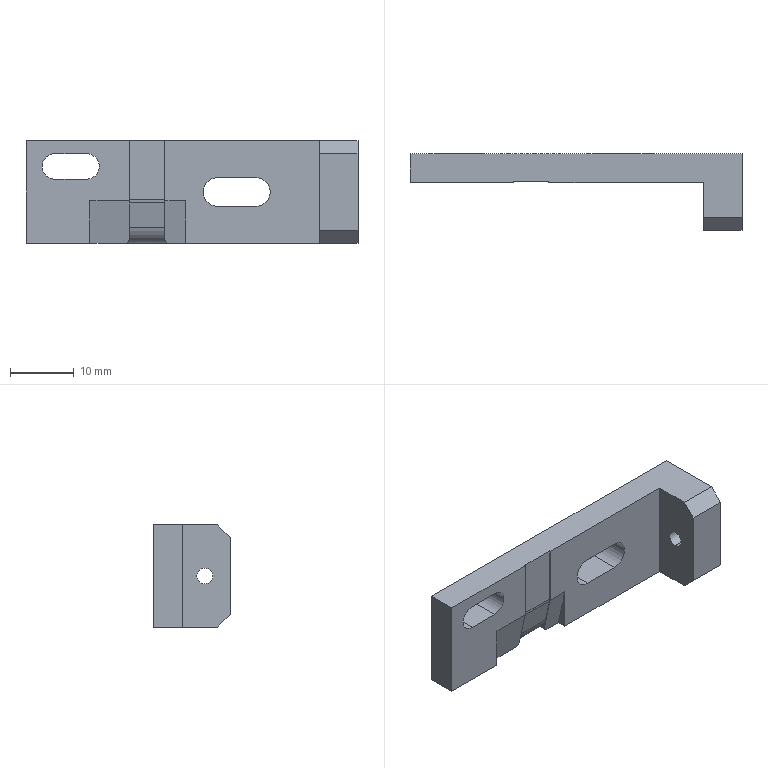Part | SolidWorks | features ICE 6, Chamfer 2, Fillet 2, 3DProfileFeature 1, Extrusion 1, HoleWzd 1 | 1 solid | 33 faces | box 52 x 12 x 16 mm | volume 3986 mm3 | plane 25 | cylinder 8 | commonest cylinder face diameters 4 x3 2.5 x2 4.5 x2 6 x1
STEP:
#1=CARTESIAN_POINT('',(23.,-3.5,1.25));
#2=VERTEX_POINT('',#1);
#3=CARTESIAN_POINT('',(23.,-3.5,-1.25));
#4=VERTEX_POINT('',#3);
#5=CARTESIAN_POINT('',(23.,-3.5,0.));
#6=DIRECTION('',(1.,0.,0.));
#7=DIRECTION('',(0.,0.,-1.));
#8=AXIS2_PLACEMENT_3D('',#5,#6,#7);
#9=CIRCLE('',#8,1.25);
#10=EDGE_CURVE('',#2,#4,#9,.T.);
#11=ORIENTED_EDGE('',*,*,#10,.F.);
#12=CARTESIAN_POINT('',(29.,-3.5,1.25));
#13=VERTEX_POINT('',#12);
#14=CARTESIAN_POINT('',(29.,-3.5,1.25));
#15=DIRECTION('',(1.,0.,0.));
#16=VECTOR('',#15,1000.);
#17=LINE('',#14,#16);
#18=EDGE_CURVE('',#2,#13,#17,.T.);
#19=ORIENTED_EDGE('',*,*,#18,.T.);
#20=CARTESIAN_POINT('',(29.,-3.5,-1.25));
#21=VERTEX_POINT('',#20);
#22=CARTESIAN_POINT('',(29.,-3.5,0.));
#23=DIRECTION('',(1.,0.,0.));
#24=DIRECTION('',(0.,0.,-1.));
#25=AXIS2_PLACEMENT_3D('',#22,#23,#24);
#26=CIRCLE('',#25,1.25);
#27=EDGE_CURVE('',#13,#21,#26,.T.);
#28=ORIENTED_EDGE('',*,*,#27,.T.);
#29=CARTESIAN_POINT('',(29.,-3.5,-1.25));
#30=DIRECTION('',(1.,0.,0.));
#31=VECTOR('',#30,1000.);
#32=LINE('',#29,#31);
#33=EDGE_CURVE('',#4,#21,#32,.T.);
#34=ORIENTED_EDGE('',*,*,#33,.F.);
#35=EDGE_LOOP('',(#11,#19,#28,#34));
#36=FACE_OUTER_BOUND('',#35,.T.);
#37=CARTESIAN_POINT('',(29.,-3.5,0.));
#38=DIRECTION('',(1.,0.,0.));
#39=DIRECTION('',(0.,0.,-1.));
#40=AXIS2_PLACEMENT_3D('',#37,#38,#39);
#41=CYLINDRICAL_SURFACE('',#40,1.25);
#42=ADVANCED_FACE('',(#36),#41,.F.);
#43=CARTESIAN_POINT('',(-13.5,0.,2.));
#44=VERTEX_POINT('',#43);
#45=CARTESIAN_POINT('',(-18.5,0.,2.));
#46=VERTEX_POINT('',#45);
#47=CARTESIAN_POINT('',(0.,0.,2.));
#48=DIRECTION('',(-1.,0.,0.));
#49=VECTOR('',#48,1000.);
#50=LINE('',#47,#49);
#51=EDGE_CURVE('',#44,#46,#50,.T.);
#52=ORIENTED_EDGE('',*,*,#51,.T.);
#53=CARTESIAN_POINT('',(-18.5,0.,6.));
#54=VERTEX_POINT('',#53);
#55=CARTESIAN_POINT('',(-18.5,0.,4.));
#56=DIRECTION('',(0.,1.,0.));
#57=DIRECTION('',(0.,0.,1.));
#58=AXIS2_PLACEMENT_3D('',#55,#56,#57);
#59=CIRCLE('',#58,2.);
#60=EDGE_CURVE('',#46,#54,#59,.T.);
#61=ORIENTED_EDGE('',*,*,#60,.T.);
#62=CARTESIAN_POINT('',(-13.5,0.,6.));
#63=VERTEX_POINT('',#62);
#64=CARTESIAN_POINT('',(0.,0.,6.));
#65=DIRECTION('',(1.,0.,0.));
#66=VECTOR('',#65,1000.);
#67=LINE('',#64,#66);
#68=EDGE_CURVE('',#54,#63,#67,.T.);
#69=ORIENTED_EDGE('',*,*,#68,.T.);
#70=CARTESIAN_POINT('',(-13.5,0.,4.));
#71=DIRECTION('',(0.,1.,0.));
#72=DIRECTION('',(0.,0.,1.));
#73=AXIS2_PLACEMENT_3D('',#70,#71,#72);
#74=CIRCLE('',#73,2.);
#75=EDGE_CURVE('',#63,#44,#74,.T.);
#76=ORIENTED_EDGE('',*,*,#75,.T.);
#77=EDGE_LOOP('',(#52,#61,#69,#76));
#78=FACE_BOUND('',#77,.T.);
#79=CARTESIAN_POINT('',(-6.75,0.,8.));
#80=VERTEX_POINT('',#79);
#81=CARTESIAN_POINT('',(-6.75,0.,-1.4));
#82=VERTEX_POINT('',#81);
#83=CARTESIAN_POINT('',(-6.75,0.,0.));
#84=DIRECTION('',(0.,0.,-1.));
#85=VECTOR('',#84,1000.);
#86=LINE('',#83,#85);
#87=EDGE_CURVE('',#80,#82,#86,.T.);
#88=ORIENTED_EDGE('',*,*,#87,.F.);
#89=CARTESIAN_POINT('',(-23.,0.,8.));
#90=VERTEX_POINT('',#89);
#91=CARTESIAN_POINT('',(-23.,0.,8.));
#92=DIRECTION('',(1.,0.,0.));
#93=VECTOR('',#92,1000.);
#94=LINE('',#91,#93);
#95=EDGE_CURVE('',#90,#80,#94,.T.);
#96=ORIENTED_EDGE('',*,*,#95,.F.);
#97=CARTESIAN_POINT('',(-23.,0.,-8.));
#98=VERTEX_POINT('',#97);
#99=CARTESIAN_POINT('',(-23.,0.,-8.));
#100=DIRECTION('',(0.,0.,1.));
#101=VECTOR('',#100,1000.);
#102=LINE('',#99,#101);
#103=EDGE_CURVE('',#98,#90,#102,.T.);
#104=ORIENTED_EDGE('',*,*,#103,.F.);
#105=CARTESIAN_POINT('',(-13.,0.,-8.));
#106=VERTEX_POINT('',#105);
#107=CARTESIAN_POINT('',(-23.,0.,-8.));
#108=DIRECTION('',(-1.,0.,0.));
#109=VECTOR('',#108,1000.);
#110=LINE('',#107,#109);
#111=EDGE_CURVE('',#106,#98,#110,.T.);
#112=ORIENTED_EDGE('',*,*,#111,.F.);
#113=CARTESIAN_POINT('',(-13.,0.,-1.4));
#114=VERTEX_POINT('',#113);
#115=CARTESIAN_POINT('',(-13.,0.,0.));
#116=DIRECTION('',(0.,0.,1.));
#117=VECTOR('',#116,1000.);
#118=LINE('',#115,#117);
#119=EDGE_CURVE('',#106,#114,#118,.T.);
#120=ORIENTED_EDGE('',*,*,#119,.T.);
#121=CARTESIAN_POINT('',(2.,0.,-1.4));
#122=DIRECTION('',(-1.,0.,0.));
#123=VECTOR('',#122,1000.);
#124=LINE('',#121,#123);
#125=EDGE_CURVE('',#82,#114,#124,.T.);
#126=ORIENTED_EDGE('',*,*,#125,.F.);
#127=EDGE_LOOP('',(#88,#96,#104,#112,#120,#126));
#128=FACE_OUTER_BOUND('',#127,.T.);
#129=CARTESIAN_POINT('',(0.,0.,0.));
#130=DIRECTION('',(0.,1.,0.));
#131=DIRECTION('',(0.,0.,1.));
#132=AXIS2_PLACEMENT_3D('',#129,#130,#131);
#133=PLANE('',#132);
#134=ADVANCED_FACE('',(#78,#128),#133,.F.);
#135=CARTESIAN_POINT('',(-7.25,1.403,-8.));
#136=VERTEX_POINT('',#135);
#137=CARTESIAN_POINT('',(-13.,1.403,-8.));
#138=VERTEX_POINT('',#137);
#139=CARTESIAN_POINT('',(-23.,1.403,-8.));
#140=DIRECTION('',(-1.,0.,0.));
#141=VECTOR('',#140,1000.);
#142=LINE('',#139,#141);
#143=EDGE_CURVE('',#136,#138,#142,.T.);
#144=ORIENTED_EDGE('',*,*,#143,.F.);
#145=CARTESIAN_POINT('',(-6.75,1.297,-7.5));
#146=VERTEX_POINT('',#145);
#147=CARTESIAN_POINT('',(-7.572,1.471,-8.322));
#148=DIRECTION('',(0.6993,-0.1486,0.6993));
#149=VECTOR('',#148,1000.);
#150=LINE('',#147,#149);
#151=EDGE_CURVE('',#136,#146,#150,.T.);
#152=ORIENTED_EDGE('',*,*,#151,.T.);
#153=CARTESIAN_POINT('',(-6.75,0.,-1.4));
#154=DIRECTION('',(0.,0.2079,-0.9781));
#155=VECTOR('',#154,1000.);
#156=LINE('',#153,#155);
#157=EDGE_CURVE('',#82,#146,#156,.T.);
#158=ORIENTED_EDGE('',*,*,#157,.F.);
#159=ORIENTED_EDGE('',*,*,#125,.T.);
#160=CARTESIAN_POINT('',(-13.,0.,-1.4));
#161=DIRECTION('',(0.,0.2079,-0.9781));
#162=VECTOR('',#161,1000.);
#163=LINE('',#160,#162);
#164=EDGE_CURVE('',#114,#138,#163,.T.);
#165=ORIENTED_EDGE('',*,*,#164,.T.);
#166=EDGE_LOOP('',(#144,#152,#158,#159,#165));
#167=FACE_OUTER_BOUND('',#166,.T.);
#168=CARTESIAN_POINT('',(2.,0.,-1.4));
#169=DIRECTION('',(0.,0.9781,0.2079));
#170=DIRECTION('',(0.,-0.2079,0.9781));
#171=AXIS2_PLACEMENT_3D('',#168,#169,#170);
#172=PLANE('',#171);
#173=ADVANCED_FACE('',(#167),#172,.F.);
#174=CARTESIAN_POINT('',(-0.75,3.934,-8.));
#175=VERTEX_POINT('',#174);
#176=CARTESIAN_POINT('',(-7.25,3.934,-8.));
#177=VERTEX_POINT('',#176);
#178=CARTESIAN_POINT('',(-23.,3.934,-8.));
#179=DIRECTION('',(-1.,0.,0.));
#180=VECTOR('',#179,1000.);
#181=LINE('',#178,#180);
#182=EDGE_CURVE('',#175,#177,#181,.T.);
#183=ORIENTED_EDGE('',*,*,#182,.T.);
#184=CARTESIAN_POINT('',(-7.25,1.403,-8.));
#185=DIRECTION('',(0.,-1.,0.));
#186=VECTOR('',#185,1000.);
#187=LINE('',#184,#186);
#188=EDGE_CURVE('',#177,#136,#187,.T.);
#189=ORIENTED_EDGE('',*,*,#188,.T.);
#190=ORIENTED_EDGE('',*,*,#143,.T.);
#191=CARTESIAN_POINT('',(-13.,4.5,-8.));
#192=DIRECTION('',(0.,-1.,0.));
#193=VECTOR('',#192,1000.);
#194=LINE('',#191,#193);
#195=EDGE_CURVE('',#138,#106,#194,.T.);
#196=ORIENTED_EDGE('',*,*,#195,.T.);
#197=ORIENTED_EDGE('',*,*,#111,.T.);
#198=CARTESIAN_POINT('',(-23.,4.5,-8.));
#199=VERTEX_POINT('',#198);
#200=CARTESIAN_POINT('',(-23.,4.5,-8.));
#201=DIRECTION('',(0.,-1.,0.));
#202=VECTOR('',#201,1000.);
#203=LINE('',#200,#202);
#204=EDGE_CURVE('',#199,#98,#203,.T.);
#205=ORIENTED_EDGE('',*,*,#204,.F.);
#206=CARTESIAN_POINT('',(29.,4.5,-8.));
#207=VERTEX_POINT('',#206);
#208=CARTESIAN_POINT('',(-23.,4.5,-8.));
#209=DIRECTION('',(-1.,0.,0.));
#210=VECTOR('',#209,1000.);
#211=LINE('',#208,#210);
#212=EDGE_CURVE('',#207,#199,#211,.T.);
#213=ORIENTED_EDGE('',*,*,#212,.F.);
#214=CARTESIAN_POINT('',(29.,-5.5,-8.));
#215=VERTEX_POINT('',#214);
#216=CARTESIAN_POINT('',(29.,4.5,-8.));
#217=DIRECTION('',(0.,1.,0.));
#218=VECTOR('',#217,1000.);
#219=LINE('',#216,#218);
#220=EDGE_CURVE('',#215,#207,#219,.T.);
#221=ORIENTED_EDGE('',*,*,#220,.F.);
#222=CARTESIAN_POINT('',(23.,-5.5,-8.));
#223=VERTEX_POINT('',#222);
#224=CARTESIAN_POINT('',(-23.,-5.5,-8.));
#225=DIRECTION('',(-1.,0.,0.));
#226=VECTOR('',#225,1000.);
#227=LINE('',#224,#226);
#228=EDGE_CURVE('',#215,#223,#227,.T.);
#229=ORIENTED_EDGE('',*,*,#228,.T.);
#230=CARTESIAN_POINT('',(23.,0.,-8.));
#231=VERTEX_POINT('',#230);
#232=CARTESIAN_POINT('',(23.,4.5,-8.));
#233=DIRECTION('',(0.,1.,0.));
#234=VECTOR('',#233,1000.);
#235=LINE('',#232,#234);
#236=EDGE_CURVE('',#223,#231,#235,.T.);
#237=ORIENTED_EDGE('',*,*,#236,.T.);
#238=CARTESIAN_POINT('',(2.,0.,-8.));
#239=VERTEX_POINT('',#238);
#240=CARTESIAN_POINT('',(-23.,0.,-8.));
#241=DIRECTION('',(-1.,0.,0.));
#242=VECTOR('',#241,1000.);
#243=LINE('',#240,#242);
#244=EDGE_CURVE('',#231,#239,#243,.T.);
#245=ORIENTED_EDGE('',*,*,#244,.T.);
#246=CARTESIAN_POINT('',(2.,1.403,-8.));
#247=VERTEX_POINT('',#246);
#248=CARTESIAN_POINT('',(2.,4.5,-8.));
#249=DIRECTION('',(0.,-1.,0.));
#250=VECTOR('',#249,1000.);
#251=LINE('',#248,#250);
#252=EDGE_CURVE('',#247,#239,#251,.T.);
#253=ORIENTED_EDGE('',*,*,#252,.F.);
#254=CARTESIAN_POINT('',(-0.75,1.403,-8.));
#255=VERTEX_POINT('',#254);
#256=CARTESIAN_POINT('',(-23.,1.403,-8.));
#257=DIRECTION('',(-1.,0.,0.));
#258=VECTOR('',#257,1000.);
#259=LINE('',#256,#258);
#260=EDGE_CURVE('',#247,#255,#259,.T.);
#261=ORIENTED_EDGE('',*,*,#260,.T.);
#262=CARTESIAN_POINT('',(-0.75,4.5,-8.));
#263=DIRECTION('',(0.,1.,0.));
#264=VECTOR('',#263,1000.);
#265=LINE('',#262,#264);
#266=EDGE_CURVE('',#255,#175,#265,.T.);
#267=ORIENTED_EDGE('',*,*,#266,.T.);
#268=EDGE_LOOP('',(#183,#189,#190,#196,#197,#205,#213,#221,#229,#237,#245,#253,#261,#267));
#269=FACE_OUTER_BOUND('',#268,.T.);
#270=CARTESIAN_POINT('',(-23.,4.5,-8.));
#271=DIRECTION('',(0.,0.,1.));
#272=DIRECTION('',(1.,0.,0.));
#273=AXIS2_PLACEMENT_3D('',#270,#271,#272);
#274=PLANE('',#273);
#275=ADVANCED_FACE('',(#269),#274,.F.);
#276=CARTESIAN_POINT('',(13.,0.,-2.25));
#277=VERTEX_POINT('',#276);
#278=CARTESIAN_POINT('',(7.,0.,-2.25));
#279=VERTEX_POINT('',#278);
#280=CARTESIAN_POINT('',(0.,0.,-2.25));
#281=DIRECTION('',(-1.,0.,0.));
#282=VECTOR('',#281,1000.);
#283=LINE('',#280,#282);
#284=EDGE_CURVE('',#277,#279,#283,.T.);
#285=ORIENTED_EDGE('',*,*,#284,.T.);
#286=CARTESIAN_POINT('',(7.,0.,2.25));
#287=VERTEX_POINT('',#286);
#288=CARTESIAN_POINT('',(7.,0.,0.));
#289=DIRECTION('',(0.,1.,0.));
#290=DIRECTION('',(0.,0.,1.));
#291=AXIS2_PLACEMENT_3D('',#288,#289,#290);
#292=CIRCLE('',#291,2.25);
#293=EDGE_CURVE('',#279,#287,#292,.T.);
#294=ORIENTED_EDGE('',*,*,#293,.T.);
#295=CARTESIAN_POINT('',(13.,0.,2.25));
#296=VERTEX_POINT('',#295);
#297=CARTESIAN_POINT('',(0.,0.,2.25));
#298=DIRECTION('',(1.,0.,0.));
#299=VECTOR('',#298,1000.);
#300=LINE('',#297,#299);
#301=EDGE_CURVE('',#287,#296,#300,.T.);
#302=ORIENTED_EDGE('',*,*,#301,.T.);
#303=CARTESIAN_POINT('',(13.,0.,0.));
#304=DIRECTION('',(0.,1.,0.));
#305=DIRECTION('',(0.,0.,1.));
#306=AXIS2_PLACEMENT_3D('',#303,#304,#305);
#307=CIRCLE('',#306,2.25);
#308=EDGE_CURVE('',#296,#277,#307,.T.);
#309=ORIENTED_EDGE('',*,*,#308,.T.);
#310=EDGE_LOOP('',(#285,#294,#302,#309));
#311=FACE_BOUND('',#310,.T.);
#312=CARTESIAN_POINT('',(-1.25,0.,8.));
#313=VERTEX_POINT('',#312);
#314=CARTESIAN_POINT('',(23.,0.,8.));
#315=VERTEX_POINT('',#314);
#316=CARTESIAN_POINT('',(-23.,0.,8.));
#317=DIRECTION('',(1.,0.,0.));
#318=VECTOR('',#317,1000.);
#319=LINE('',#316,#318);
#320=EDGE_CURVE('',#313,#315,#319,.T.);
#321=ORIENTED_EDGE('',*,*,#320,.F.);
#322=CARTESIAN_POINT('',(-1.25,0.,-1.4));
#323=VERTEX_POINT('',#322);
#324=CARTESIAN_POINT('',(-1.25,0.,0.));
#325=DIRECTION('',(0.,0.,-1.));
#326=VECTOR('',#325,1000.);
#327=LINE('',#324,#326);
#328=EDGE_CURVE('',#313,#323,#327,.T.);
#329=ORIENTED_EDGE('',*,*,#328,.T.);
#330=CARTESIAN_POINT('',(2.,0.,-1.4));
#331=VERTEX_POINT('',#330);
#332=CARTESIAN_POINT('',(2.,0.,-1.4));
#333=DIRECTION('',(-1.,0.,0.));
#334=VECTOR('',#333,1000.);
#335=LINE('',#332,#334);
#336=EDGE_CURVE('',#331,#323,#335,.T.);
#337=ORIENTED_EDGE('',*,*,#336,.F.);
#338=CARTESIAN_POINT('',(2.,0.,0.));
#339=DIRECTION('',(0.,0.,1.));
#340=VECTOR('',#339,1000.);
#341=LINE('',#338,#340);
#342=EDGE_CURVE('',#239,#331,#341,.T.);
#343=ORIENTED_EDGE('',*,*,#342,.F.);
#344=ORIENTED_EDGE('',*,*,#244,.F.);
#345=CARTESIAN_POINT('',(23.,0.,-8.));
#346=DIRECTION('',(0.,0.,-1.));
#347=VECTOR('',#346,1000.);
#348=LINE('',#345,#347);
#349=EDGE_CURVE('',#315,#231,#348,.T.);
#350=ORIENTED_EDGE('',*,*,#349,.F.);
#351=EDGE_LOOP('',(#321,#329,#337,#343,#344,#350));
#352=FACE_OUTER_BOUND('',#351,.T.);
#353=CARTESIAN_POINT('',(0.,0.,0.));
#354=DIRECTION('',(0.,1.,0.));
#355=DIRECTION('',(0.,0.,1.));
#356=AXIS2_PLACEMENT_3D('',#353,#354,#355);
#357=PLANE('',#356);
#358=ADVANCED_FACE('',(#311,#352),#357,.F.);
#359=ORIENTED_EDGE('',*,*,#103,.T.);
#360=CARTESIAN_POINT('',(-23.,4.5,8.));
#361=VERTEX_POINT('',#360);
#362=CARTESIAN_POINT('',(-23.,4.5,8.));
#363=DIRECTION('',(0.,-1.,0.));
#364=VECTOR('',#363,1000.);
#365=LINE('',#362,#364);
#366=EDGE_CURVE('',#361,#90,#365,.T.);
#367=ORIENTED_EDGE('',*,*,#366,.F.);
#368=CARTESIAN_POINT('',(-23.,4.5,-8.));
#369=DIRECTION('',(0.,0.,1.));
#370=VECTOR('',#369,1000.);
#371=LINE('',#368,#370);
#372=EDGE_CURVE('',#199,#361,#371,.T.);
#373=ORIENTED_EDGE('',*,*,#372,.F.);
#374=ORIENTED_EDGE('',*,*,#204,.T.);
#375=EDGE_LOOP('',(#359,#367,#373,#374));
#376=FACE_OUTER_BOUND('',#375,.T.);
#377=CARTESIAN_POINT('',(-23.,4.5,-8.));
#378=DIRECTION('',(1.,0.,0.));
#379=DIRECTION('',(0.,0.,-1.));
#380=AXIS2_PLACEMENT_3D('',#377,#378,#379);
#381=PLANE('',#380);
#382=ADVANCED_FACE('',(#376),#381,.F.);
#383=CARTESIAN_POINT('',(-1.25,0.1,8.));
#384=VERTEX_POINT('',#383);
#385=CARTESIAN_POINT('',(-6.75,0.1,8.));
#386=VERTEX_POINT('',#385);
#387=CARTESIAN_POINT('',(-1.25,0.1,8.));
#388=DIRECTION('',(-1.,0.,0.));
#389=VECTOR('',#388,1000.);
#390=LINE('',#387,#389);
#391=EDGE_CURVE('',#384,#386,#390,.T.);
#392=ORIENTED_EDGE('',*,*,#391,.F.);
#393=CARTESIAN_POINT('',(-1.25,0.1,8.));
#394=DIRECTION('',(0.,1.,0.));
#395=VECTOR('',#394,1000.);
#396=LINE('',#393,#395);
#397=EDGE_CURVE('',#313,#384,#396,.T.);
#398=ORIENTED_EDGE('',*,*,#397,.F.);
#399=ORIENTED_EDGE('',*,*,#320,.T.);
#400=CARTESIAN_POINT('',(23.,-5.5,8.));
#401=VERTEX_POINT('',#400);
#402=CARTESIAN_POINT('',(23.,4.5,8.));
#403=DIRECTION('',(0.,-1.,0.));
#404=VECTOR('',#403,1000.);
#405=LINE('',#402,#404);
#406=EDGE_CURVE('',#315,#401,#405,.T.);
#407=ORIENTED_EDGE('',*,*,#406,.T.);
#408=CARTESIAN_POINT('',(29.,-5.5,8.));
#409=VERTEX_POINT('',#408);
#410=CARTESIAN_POINT('',(-23.,-5.5,8.));
#411=DIRECTION('',(1.,0.,0.));
#412=VECTOR('',#411,1000.);
#413=LINE('',#410,#412);
#414=EDGE_CURVE('',#401,#409,#413,.T.);
#415=ORIENTED_EDGE('',*,*,#414,.T.);
#416=CARTESIAN_POINT('',(29.,4.5,8.));
#417=VERTEX_POINT('',#416);
#418=CARTESIAN_POINT('',(29.,4.5,8.));
#419=DIRECTION('',(0.,-1.,0.));
#420=VECTOR('',#419,1000.);
#421=LINE('',#418,#420);
#422=EDGE_CURVE('',#417,#409,#421,.T.);
#423=ORIENTED_EDGE('',*,*,#422,.F.);
#424=CARTESIAN_POINT('',(-23.,4.5,8.));
#425=DIRECTION('',(1.,0.,0.));
#426=VECTOR('',#425,1000.);
#427=LINE('',#424,#426);
#428=EDGE_CURVE('',#361,#417,#427,.T.);
#429=ORIENTED_EDGE('',*,*,#428,.F.);
#430=ORIENTED_EDGE('',*,*,#366,.T.);
#431=ORIENTED_EDGE('',*,*,#95,.T.);
#432=CARTESIAN_POINT('',(-6.75,0.1,8.));
#433=DIRECTION('',(0.,1.,0.));
#434=VECTOR('',#433,1000.);
#435=LINE('',#432,#434);
#436=EDGE_CURVE('',#80,#386,#435,.T.);
#437=ORIENTED_EDGE('',*,*,#436,.T.);
#438=EDGE_LOOP('',(#392,#398,#399,#407,#415,#423,#429,#430,#431,#437));
#439=FACE_OUTER_BOUND('',#438,.T.);
#440=CARTESIAN_POINT('',(-23.,4.5,8.));
#441=DIRECTION('',(0.,0.,-1.));
#442=DIRECTION('',(-1.,0.,0.));
#443=AXIS2_PLACEMENT_3D('',#440,#441,#442);
#444=PLANE('',#443);
#445=ADVANCED_FACE('',(#439),#444,.F.);
#446=CARTESIAN_POINT('',(7.,4.5,-2.25));
#447=VERTEX_POINT('',#446);
#448=CARTESIAN_POINT('',(7.,4.5,2.25));
#449=VERTEX_POINT('',#448);
#450=CARTESIAN_POINT('',(7.,4.5,0.));
#451=DIRECTION('',(0.,1.,0.));
#452=DIRECTION('',(0.,0.,1.));
#453=AXIS2_PLACEMENT_3D('',#450,#451,#452);
#454=CIRCLE('',#453,2.25);
#455=EDGE_CURVE('',#447,#449,#454,.T.);
#456=ORIENTED_EDGE('',*,*,#455,.F.);
#457=CARTESIAN_POINT('',(13.,4.5,-2.25));
#458=VERTEX_POINT('',#457);
#459=CARTESIAN_POINT('',(7.,4.5,-2.25));
#460=DIRECTION('',(-1.,0.,0.));
#461=VECTOR('',#460,1000.);
#462=LINE('',#459,#461);
#463=EDGE_CURVE('',#458,#447,#462,.T.);
#464=ORIENTED_EDGE('',*,*,#463,.F.);
#465=CARTESIAN_POINT('',(13.,4.5,2.25));
#466=VERTEX_POINT('',#465);
#467=CARTESIAN_POINT('',(13.,4.5,0.));
#468=DIRECTION('',(0.,1.,0.));
#469=DIRECTION('',(0.,0.,1.));
#470=AXIS2_PLACEMENT_3D('',#467,#468,#469);
#471=CIRCLE('',#470,2.25);
#472=EDGE_CURVE('',#466,#458,#471,.T.);
#473=ORIENTED_EDGE('',*,*,#472,.F.);
#474=CARTESIAN_POINT('',(7.,4.5,2.25));
#475=DIRECTION('',(1.,0.,0.));
#476=VECTOR('',#475,1000.);
#477=LINE('',#474,#476);
#478=EDGE_CURVE('',#449,#466,#477,.T.);
#479=ORIENTED_EDGE('',*,*,#478,.F.);
#480=EDGE_LOOP('',(#456,#464,#473,#479));
#481=FACE_BOUND('',#480,.T.);
#482=CARTESIAN_POINT('',(-18.5,4.5,2.));
#483=VERTEX_POINT('',#482);
#484=CARTESIAN_POINT('',(-18.5,4.5,6.));
#485=VERTEX_POINT('',#484);
#486=CARTESIAN_POINT('',(-18.5,4.5,4.));
#487=DIRECTION('',(0.,1.,0.));
#488=DIRECTION('',(0.,0.,1.));
#489=AXIS2_PLACEMENT_3D('',#486,#487,#488);
#490=CIRCLE('',#489,2.);
#491=EDGE_CURVE('',#483,#485,#490,.T.);
#492=ORIENTED_EDGE('',*,*,#491,.F.);
#493=CARTESIAN_POINT('',(-13.5,4.5,2.));
#494=VERTEX_POINT('',#493);
#495=CARTESIAN_POINT('',(-18.5,4.5,2.));
#496=DIRECTION('',(-1.,0.,0.));
#497=VECTOR('',#496,1000.);
#498=LINE('',#495,#497);
#499=EDGE_CURVE('',#494,#483,#498,.T.);
#500=ORIENTED_EDGE('',*,*,#499,.F.);
#501=CARTESIAN_POINT('',(-13.5,4.5,6.));
#502=VERTEX_POINT('',#501);
#503=CARTESIAN_POINT('',(-13.5,4.5,4.));
#504=DIRECTION('',(0.,1.,0.));
#505=DIRECTION('',(0.,0.,1.));
#506=AXIS2_PLACEMENT_3D('',#503,#504,#505);
#507=CIRCLE('',#506,2.);
#508=EDGE_CURVE('',#502,#494,#507,.T.);
#509=ORIENTED_EDGE('',*,*,#508,.F.);
#510=CARTESIAN_POINT('',(-18.5,4.5,6.));
#511=DIRECTION('',(1.,0.,0.));
#512=VECTOR('',#511,1000.);
#513=LINE('',#510,#512);
#514=EDGE_CURVE('',#485,#502,#513,.T.);
#515=ORIENTED_EDGE('',*,*,#514,.F.);
#516=EDGE_LOOP('',(#492,#500,#509,#515));
#517=FACE_BOUND('',#516,.T.);
#518=ORIENTED_EDGE('',*,*,#428,.T.);
#519=CARTESIAN_POINT('',(29.,4.5,8.));
#520=DIRECTION('',(0.,0.,1.));
#521=VECTOR('',#520,1000.);
#522=LINE('',#519,#521);
#523=EDGE_CURVE('',#207,#417,#522,.T.);
#524=ORIENTED_EDGE('',*,*,#523,.F.);
#525=ORIENTED_EDGE('',*,*,#212,.T.);
#526=ORIENTED_EDGE('',*,*,#372,.T.);
#527=EDGE_LOOP('',(#518,#524,#525,#526));
#528=FACE_OUTER_BOUND('',#527,.T.);
#529=CARTESIAN_POINT('',(0.,4.5,0.));
#530=DIRECTION('',(0.,1.,0.));
#531=DIRECTION('',(0.,0.,1.));
#532=AXIS2_PLACEMENT_3D('',#529,#530,#531);
#533=PLANE('',#532);
#534=ADVANCED_FACE('',(#481,#517,#528),#533,.T.);
#535=CARTESIAN_POINT('',(23.,-3.5,0.));
#536=DIRECTION('',(1.,0.,0.));
#537=DIRECTION('',(0.,0.,-1.));
#538=AXIS2_PLACEMENT_3D('',#535,#536,#537);
#539=CIRCLE('',#538,1.25);
#540=EDGE_CURVE('',#4,#2,#539,.T.);
#541=ORIENTED_EDGE('',*,*,#540,.T.);
#542=ORIENTED_EDGE('',*,*,#10,.T.);
#543=EDGE_LOOP('',(#541,#542));
#544=FACE_BOUND('',#543,.T.);
#545=ORIENTED_EDGE('',*,*,#236,.F.);
#546=CARTESIAN_POINT('',(23.,-7.5,-6.));
#547=VERTEX_POINT('',#546);
#548=CARTESIAN_POINT('',(23.,-5.5,-8.));
#549=DIRECTION('',(0.,-0.7071,0.7071));
#550=VECTOR('',#549,1000.);
#551=LINE('',#548,#550);
#552=EDGE_CURVE('',#223,#547,#551,.T.);
#553=ORIENTED_EDGE('',*,*,#552,.T.);
#554=CARTESIAN_POINT('',(23.,-7.5,6.));
#555=VERTEX_POINT('',#554);
#556=CARTESIAN_POINT('',(23.,-7.5,8.));
#557=DIRECTION('',(0.,0.,-1.));
#558=VECTOR('',#557,1000.);
#559=LINE('',#556,#558);
#560=EDGE_CURVE('',#555,#547,#559,.T.);
#561=ORIENTED_EDGE('',*,*,#560,.F.);
#562=CARTESIAN_POINT('',(23.,-7.5,6.));
#563=DIRECTION('',(0.,0.7071,0.7071));
#564=VECTOR('',#563,1000.);
#565=LINE('',#562,#564);
#566=EDGE_CURVE('',#555,#401,#565,.T.);
#567=ORIENTED_EDGE('',*,*,#566,.T.);
#568=ORIENTED_EDGE('',*,*,#406,.F.);
#569=ORIENTED_EDGE('',*,*,#349,.T.);
#570=EDGE_LOOP('',(#545,#553,#561,#567,#568,#569));
#571=FACE_OUTER_BOUND('',#570,.T.);
#572=CARTESIAN_POINT('',(23.,0.,0.));
#573=DIRECTION('',(1.,0.,0.));
#574=DIRECTION('',(0.,0.,-1.));
#575=AXIS2_PLACEMENT_3D('',#572,#573,#574);
#576=PLANE('',#575);
#577=ADVANCED_FACE('',(#544,#571),#576,.F.);
#578=ORIENTED_EDGE('',*,*,#560,.T.);
#579=CARTESIAN_POINT('',(29.,-7.5,-6.));
#580=VERTEX_POINT('',#579);
#581=CARTESIAN_POINT('',(29.,-7.5,-6.));
#582=DIRECTION('',(1.,0.,0.));
#583=VECTOR('',#582,1000.);
#584=LINE('',#581,#583);
#585=EDGE_CURVE('',#547,#580,#584,.T.);
#586=ORIENTED_EDGE('',*,*,#585,.T.);
#587=CARTESIAN_POINT('',(29.,-7.5,6.));
#588=VERTEX_POINT('',#587);
#589=CARTESIAN_POINT('',(29.,-7.5,8.));
#590=DIRECTION('',(0.,0.,-1.));
#591=VECTOR('',#590,1000.);
#592=LINE('',#589,#591);
#593=EDGE_CURVE('',#588,#580,#592,.T.);
#594=ORIENTED_EDGE('',*,*,#593,.F.);
#595=CARTESIAN_POINT('',(29.,-7.5,6.));
#596=DIRECTION('',(-1.,0.,0.));
#597=VECTOR('',#596,1000.);
#598=LINE('',#595,#597);
#599=EDGE_CURVE('',#588,#555,#598,.T.);
#600=ORIENTED_EDGE('',*,*,#599,.T.);
#601=EDGE_LOOP('',(#578,#586,#594,#600));
#602=FACE_OUTER_BOUND('',#601,.T.);
#603=CARTESIAN_POINT('',(29.,-7.5,8.));
#604=DIRECTION('',(0.,1.,0.));
#605=DIRECTION('',(0.,0.,1.));
#606=AXIS2_PLACEMENT_3D('',#603,#604,#605);
#607=PLANE('',#606);
#608=ADVANCED_FACE('',(#602),#607,.F.);
#609=CARTESIAN_POINT('',(29.,-3.5,0.));
#610=DIRECTION('',(1.,0.,0.));
#611=DIRECTION('',(0.,0.,-1.));
#612=AXIS2_PLACEMENT_3D('',#609,#610,#611);
#613=CIRCLE('',#612,1.25);
#614=EDGE_CURVE('',#21,#13,#613,.T.);
#615=ORIENTED_EDGE('',*,*,#614,.F.);
#616=ORIENTED_EDGE('',*,*,#27,.F.);
#617=EDGE_LOOP('',(#615,#616));
#618=FACE_BOUND('',#617,.T.);
#619=ORIENTED_EDGE('',*,*,#593,.T.);
#620=CARTESIAN_POINT('',(29.,-6.75,-6.75));
#621=DIRECTION('',(0.,0.7071,-0.7071));
#622=VECTOR('',#621,1000.);
#623=LINE('',#620,#622);
#624=EDGE_CURVE('',#580,#215,#623,.T.);
#625=ORIENTED_EDGE('',*,*,#624,.T.);
#626=ORIENTED_EDGE('',*,*,#220,.T.);
#627=ORIENTED_EDGE('',*,*,#523,.T.);
#628=ORIENTED_EDGE('',*,*,#422,.T.);
#629=CARTESIAN_POINT('',(29.,-6.75,6.75));
#630=DIRECTION('',(0.,-0.7071,-0.7071));
#631=VECTOR('',#630,1000.);
#632=LINE('',#629,#631);
#633=EDGE_CURVE('',#409,#588,#632,.T.);
#634=ORIENTED_EDGE('',*,*,#633,.T.);
#635=EDGE_LOOP('',(#619,#625,#626,#627,#628,#634));
#636=FACE_OUTER_BOUND('',#635,.T.);
#637=CARTESIAN_POINT('',(29.,0.,0.));
#638=DIRECTION('',(1.,0.,0.));
#639=DIRECTION('',(0.,0.,-1.));
#640=AXIS2_PLACEMENT_3D('',#637,#638,#639);
#641=PLANE('',#640);
#642=ADVANCED_FACE('',(#618,#636),#641,.T.);
#643=ORIENTED_EDGE('',*,*,#18,.F.);
#644=ORIENTED_EDGE('',*,*,#540,.F.);
#645=ORIENTED_EDGE('',*,*,#33,.T.);
#646=ORIENTED_EDGE('',*,*,#614,.T.);
#647=EDGE_LOOP('',(#643,#644,#645,#646));
#648=FACE_OUTER_BOUND('',#647,.T.);
#649=CARTESIAN_POINT('',(29.,-3.5,0.));
#650=DIRECTION('',(1.,0.,0.));
#651=DIRECTION('',(0.,0.,-1.));
#652=AXIS2_PLACEMENT_3D('',#649,#650,#651);
#653=CYLINDRICAL_SURFACE('',#652,1.25);
#654=ADVANCED_FACE('',(#648),#653,.F.);
#655=ORIENTED_EDGE('',*,*,#624,.F.);
#656=ORIENTED_EDGE('',*,*,#585,.F.);
#657=ORIENTED_EDGE('',*,*,#552,.F.);
#658=ORIENTED_EDGE('',*,*,#228,.F.);
#659=EDGE_LOOP('',(#655,#656,#657,#658));
#660=FACE_OUTER_BOUND('',#659,.T.);
#661=CARTESIAN_POINT('',(-23.,-5.5,-8.));
#662=DIRECTION('',(0.,0.7071,0.7071));
#663=DIRECTION('',(-1.,0.,0.));
#664=AXIS2_PLACEMENT_3D('',#661,#662,#663);
#665=PLANE('',#664);
#666=ADVANCED_FACE('',(#660),#665,.F.);
#667=ORIENTED_EDGE('',*,*,#633,.F.);
#668=ORIENTED_EDGE('',*,*,#414,.F.);
#669=ORIENTED_EDGE('',*,*,#566,.F.);
#670=ORIENTED_EDGE('',*,*,#599,.F.);
#671=EDGE_LOOP('',(#667,#668,#669,#670));
#672=FACE_OUTER_BOUND('',#671,.T.);
#673=CARTESIAN_POINT('',(29.,-7.5,6.));
#674=DIRECTION('',(0.,0.7071,-0.7071));
#675=DIRECTION('',(-1.,0.,0.));
#676=AXIS2_PLACEMENT_3D('',#673,#674,#675);
#677=PLANE('',#676);
#678=ADVANCED_FACE('',(#672),#677,.F.);
#679=CARTESIAN_POINT('',(-1.25,1.297,-7.5));
#680=VERTEX_POINT('',#679);
#681=CARTESIAN_POINT('',(-1.25,0.,-1.4));
#682=DIRECTION('',(0.,0.2079,-0.9781));
#683=VECTOR('',#682,1000.);
#684=LINE('',#681,#683);
#685=EDGE_CURVE('',#323,#680,#684,.T.);
#686=ORIENTED_EDGE('',*,*,#685,.T.);
#687=CARTESIAN_POINT('',(-1.385,1.268,-7.365));
#688=DIRECTION('',(0.6993,0.1486,-0.6993));
#689=VECTOR('',#688,1000.);
#690=LINE('',#687,#689);
#691=EDGE_CURVE('',#680,#255,#690,.T.);
#692=ORIENTED_EDGE('',*,*,#691,.T.);
#693=ORIENTED_EDGE('',*,*,#260,.F.);
#694=CARTESIAN_POINT('',(2.,0.,-1.4));
#695=DIRECTION('',(0.,0.2079,-0.9781));
#696=VECTOR('',#695,1000.);
#697=LINE('',#694,#696);
#698=EDGE_CURVE('',#331,#247,#697,.T.);
#699=ORIENTED_EDGE('',*,*,#698,.F.);
#700=ORIENTED_EDGE('',*,*,#336,.T.);
#701=EDGE_LOOP('',(#686,#692,#693,#699,#700));
#702=FACE_OUTER_BOUND('',#701,.T.);
#703=CARTESIAN_POINT('',(2.,0.,-1.4));
#704=DIRECTION('',(0.,0.9781,0.2079));
#705=DIRECTION('',(0.,-0.2079,0.9781));
#706=AXIS2_PLACEMENT_3D('',#703,#704,#705);
#707=PLANE('',#706);
#708=ADVANCED_FACE('',(#702),#707,.F.);
#709=ORIENTED_EDGE('',*,*,#252,.T.);
#710=ORIENTED_EDGE('',*,*,#342,.T.);
#711=ORIENTED_EDGE('',*,*,#698,.T.);
#712=EDGE_LOOP('',(#709,#710,#711));
#713=FACE_OUTER_BOUND('',#712,.T.);
#714=CARTESIAN_POINT('',(2.,0.,0.));
#715=DIRECTION('',(-1.,0.,0.));
#716=DIRECTION('',(0.,0.,1.));
#717=AXIS2_PLACEMENT_3D('',#714,#715,#716);
#718=PLANE('',#717);
#719=ADVANCED_FACE('',(#713),#718,.T.);
#720=ORIENTED_EDGE('',*,*,#164,.F.);
#721=ORIENTED_EDGE('',*,*,#119,.F.);
#722=ORIENTED_EDGE('',*,*,#195,.F.);
#723=EDGE_LOOP('',(#720,#721,#722));
#724=FACE_OUTER_BOUND('',#723,.T.);
#725=CARTESIAN_POINT('',(-13.,0.,0.));
#726=DIRECTION('',(-1.,0.,0.));
#727=DIRECTION('',(0.,0.,1.));
#728=AXIS2_PLACEMENT_3D('',#725,#726,#727);
#729=PLANE('',#728);
#730=ADVANCED_FACE('',(#724),#729,.F.);
#731=CARTESIAN_POINT('',(-1.25,1.,-5.624));
#732=VERTEX_POINT('',#731);
#733=CARTESIAN_POINT('',(-1.25,2.276,-7.5));
#734=VERTEX_POINT('',#733);
#735=CARTESIAN_POINT('',(-1.25,3.934,-5.));
#736=DIRECTION('',(1.,0.,0.));
#737=DIRECTION('',(0.,0.,-1.));
#738=AXIS2_PLACEMENT_3D('',#735,#736,#737);
#739=CIRCLE('',#738,3.);
#740=EDGE_CURVE('',#732,#734,#739,.T.);
#741=ORIENTED_EDGE('',*,*,#740,.T.);
#742=CARTESIAN_POINT('',(-1.25,0.,-7.5));
#743=DIRECTION('',(0.,-1.,0.));
#744=VECTOR('',#743,1000.);
#745=LINE('',#742,#744);
#746=EDGE_CURVE('',#734,#680,#745,.T.);
#747=ORIENTED_EDGE('',*,*,#746,.T.);
#748=ORIENTED_EDGE('',*,*,#685,.F.);
#749=ORIENTED_EDGE('',*,*,#328,.F.);
#750=ORIENTED_EDGE('',*,*,#397,.T.);
#751=CARTESIAN_POINT('',(-1.25,0.1,-1.179));
#752=VERTEX_POINT('',#751);
#753=CARTESIAN_POINT('',(-1.25,0.1,8.));
#754=DIRECTION('',(0.,0.,-1.));
#755=VECTOR('',#754,1000.);
#756=LINE('',#753,#755);
#757=EDGE_CURVE('',#384,#752,#756,.T.);
#758=ORIENTED_EDGE('',*,*,#757,.T.);
#759=CARTESIAN_POINT('',(-1.25,0.1437,-1.595));
#760=VERTEX_POINT('',#759);
#761=CARTESIAN_POINT('',(-1.25,2.1,-1.179));
#762=DIRECTION('',(1.,0.,0.));
#763=DIRECTION('',(0.,0.,-1.));
#764=AXIS2_PLACEMENT_3D('',#761,#762,#763);
#765=CIRCLE('',#764,2.);
#766=EDGE_CURVE('',#752,#760,#765,.T.);
#767=ORIENTED_EDGE('',*,*,#766,.T.);
#768=CARTESIAN_POINT('',(-1.25,0.1,-1.389));
#769=DIRECTION('',(0.,0.2079,-0.9781));
#770=VECTOR('',#769,1000.);
#771=LINE('',#768,#770);
#772=EDGE_CURVE('',#760,#732,#771,.T.);
#773=ORIENTED_EDGE('',*,*,#772,.T.);
#774=EDGE_LOOP('',(#741,#747,#748,#749,#750,#758,#767,#773));
#775=FACE_OUTER_BOUND('',#774,.T.);
#776=CARTESIAN_POINT('',(-1.25,0.,0.));
#777=DIRECTION('',(1.,0.,0.));
#778=DIRECTION('',(0.,0.,-1.));
#779=AXIS2_PLACEMENT_3D('',#776,#777,#778);
#780=PLANE('',#779);
#781=ADVANCED_FACE('',(#775),#780,.F.);
#782=ORIENTED_EDGE('',*,*,#157,.T.);
#783=CARTESIAN_POINT('',(-6.75,2.276,-7.5));
#784=VERTEX_POINT('',#783);
#785=CARTESIAN_POINT('',(-6.75,3.934,-7.5));
#786=DIRECTION('',(0.,1.,0.));
#787=VECTOR('',#786,1000.);
#788=LINE('',#785,#787);
#789=EDGE_CURVE('',#146,#784,#788,.T.);
#790=ORIENTED_EDGE('',*,*,#789,.T.);
#791=CARTESIAN_POINT('',(-6.75,1.,-5.624));
#792=VERTEX_POINT('',#791);
#793=CARTESIAN_POINT('',(-6.75,3.934,-5.));
#794=DIRECTION('',(-1.,0.,0.));
#795=DIRECTION('',(0.,0.,-1.));
#796=AXIS2_PLACEMENT_3D('',#793,#794,#795);
#797=CIRCLE('',#796,3.);
#798=EDGE_CURVE('',#784,#792,#797,.T.);
#799=ORIENTED_EDGE('',*,*,#798,.T.);
#800=CARTESIAN_POINT('',(-6.75,0.1437,-1.595));
#801=VERTEX_POINT('',#800);
#802=CARTESIAN_POINT('',(-6.75,0.1,-1.389));
#803=DIRECTION('',(0.,0.2079,-0.9781));
#804=VECTOR('',#803,1000.);
#805=LINE('',#802,#804);
#806=EDGE_CURVE('',#801,#792,#805,.T.);
#807=ORIENTED_EDGE('',*,*,#806,.F.);
#808=CARTESIAN_POINT('',(-6.75,0.1,-1.179));
#809=VERTEX_POINT('',#808);
#810=CARTESIAN_POINT('',(-6.75,2.1,-1.179));
#811=DIRECTION('',(-1.,0.,0.));
#812=DIRECTION('',(0.,0.,-1.));
#813=AXIS2_PLACEMENT_3D('',#810,#811,#812);
#814=CIRCLE('',#813,2.);
#815=EDGE_CURVE('',#801,#809,#814,.T.);
#816=ORIENTED_EDGE('',*,*,#815,.T.);
#817=CARTESIAN_POINT('',(-6.75,0.1,8.));
#818=DIRECTION('',(0.,0.,-1.));
#819=VECTOR('',#818,1000.);
#820=LINE('',#817,#819);
#821=EDGE_CURVE('',#386,#809,#820,.T.);
#822=ORIENTED_EDGE('',*,*,#821,.F.);
#823=ORIENTED_EDGE('',*,*,#436,.F.);
#824=ORIENTED_EDGE('',*,*,#87,.T.);
#825=EDGE_LOOP('',(#782,#790,#799,#807,#816,#822,#823,#824));
#826=FACE_OUTER_BOUND('',#825,.T.);
#827=CARTESIAN_POINT('',(-6.75,0.,0.));
#828=DIRECTION('',(1.,0.,0.));
#829=DIRECTION('',(0.,0.,-1.));
#830=AXIS2_PLACEMENT_3D('',#827,#828,#829);
#831=PLANE('',#830);
#832=ADVANCED_FACE('',(#826),#831,.T.);
#833=ORIENTED_EDGE('',*,*,#821,.T.);
#834=CARTESIAN_POINT('',(-1.25,0.1,-1.179));
#835=DIRECTION('',(1.,0.,0.));
#836=VECTOR('',#835,1000.);
#837=LINE('',#834,#836);
#838=EDGE_CURVE('',#809,#752,#837,.T.);
#839=ORIENTED_EDGE('',*,*,#838,.T.);
#840=ORIENTED_EDGE('',*,*,#757,.F.);
#841=ORIENTED_EDGE('',*,*,#391,.T.);
#842=EDGE_LOOP('',(#833,#839,#840,#841));
#843=FACE_OUTER_BOUND('',#842,.T.);
#844=CARTESIAN_POINT('',(-1.25,0.1,8.));
#845=DIRECTION('',(0.,1.,0.));
#846=DIRECTION('',(0.,0.,1.));
#847=AXIS2_PLACEMENT_3D('',#844,#845,#846);
#848=PLANE('',#847);
#849=ADVANCED_FACE('',(#843),#848,.F.);
#850=ORIENTED_EDGE('',*,*,#772,.F.);
#851=CARTESIAN_POINT('',(-1.25,0.1437,-1.595));
#852=DIRECTION('',(-1.,0.,0.));
#853=VECTOR('',#852,1000.);
#854=LINE('',#851,#853);
#855=EDGE_CURVE('',#760,#801,#854,.T.);
#856=ORIENTED_EDGE('',*,*,#855,.T.);
#857=ORIENTED_EDGE('',*,*,#806,.T.);
#858=CARTESIAN_POINT('',(-1.25,1.,-5.624));
#859=DIRECTION('',(1.,0.,0.));
#860=VECTOR('',#859,1000.);
#861=LINE('',#858,#860);
#862=EDGE_CURVE('',#792,#732,#861,.T.);
#863=ORIENTED_EDGE('',*,*,#862,.T.);
#864=EDGE_LOOP('',(#850,#856,#857,#863));
#865=FACE_OUTER_BOUND('',#864,.T.);
#866=CARTESIAN_POINT('',(-1.25,0.1,-1.389));
#867=DIRECTION('',(0.,0.9781,0.2079));
#868=DIRECTION('',(0.,-0.2079,0.9781));
#869=AXIS2_PLACEMENT_3D('',#866,#867,#868);
#870=PLANE('',#869);
#871=ADVANCED_FACE('',(#865),#870,.F.);
#872=ORIENTED_EDGE('',*,*,#740,.F.);
#873=ORIENTED_EDGE('',*,*,#862,.F.);
#874=ORIENTED_EDGE('',*,*,#798,.F.);
#875=CARTESIAN_POINT('',(-6.75,2.276,-7.5));
#876=CARTESIAN_POINT('',(-7.078,2.771,-7.828));
#877=CARTESIAN_POINT('',(-7.25,3.34,-8.));
#878=CARTESIAN_POINT('',(-7.25,3.934,-8.));
#879=(BOUNDED_CURVE()B_SPLINE_CURVE(3,(#875,#876,#877,#878),.UNSPECIFIED.,.F.,.F.)B_SPLINE_CURVE_WITH_KNOTS((4,4),(5.697,6.283),.UNSPECIFIED.)CURVE()GEOMETRIC_REPRESENTATION_ITEM()RATIONAL_B_SPLINE_CURVE((1.,0.9716,0.9716,1.))REPRESENTATION_ITEM(''));
#880=EDGE_CURVE('',#784,#177,#879,.T.);
#881=ORIENTED_EDGE('',*,*,#880,.T.);
#882=ORIENTED_EDGE('',*,*,#182,.F.);
#883=CARTESIAN_POINT('',(-0.75,3.934,-8.));
#884=CARTESIAN_POINT('',(-0.75,3.34,-8.));
#885=CARTESIAN_POINT('',(-0.9215,2.771,-7.828));
#886=CARTESIAN_POINT('',(-1.25,2.276,-7.5));
#887=(BOUNDED_CURVE()B_SPLINE_CURVE(3,(#883,#884,#885,#886),.UNSPECIFIED.,.F.,.F.)B_SPLINE_CURVE_WITH_KNOTS((4,4),(3.142,3.727),.UNSPECIFIED.)CURVE()GEOMETRIC_REPRESENTATION_ITEM()RATIONAL_B_SPLINE_CURVE((1.,0.9716,0.9716,1.))REPRESENTATION_ITEM(''));
#888=EDGE_CURVE('',#175,#734,#887,.T.);
#889=ORIENTED_EDGE('',*,*,#888,.T.);
#890=EDGE_LOOP('',(#872,#873,#874,#881,#882,#889));
#891=FACE_OUTER_BOUND('',#890,.T.);
#892=CARTESIAN_POINT('',(-23.,3.934,-5.));
#893=DIRECTION('',(-1.,0.,0.));
#894=DIRECTION('',(0.,0.,1.));
#895=AXIS2_PLACEMENT_3D('',#892,#893,#894);
#896=CYLINDRICAL_SURFACE('',#895,3.);
#897=ADVANCED_FACE('',(#891),#896,.T.);
#898=ORIENTED_EDGE('',*,*,#766,.F.);
#899=ORIENTED_EDGE('',*,*,#838,.F.);
#900=ORIENTED_EDGE('',*,*,#815,.F.);
#901=ORIENTED_EDGE('',*,*,#855,.F.);
#902=EDGE_LOOP('',(#898,#899,#900,#901));
#903=FACE_OUTER_BOUND('',#902,.T.);
#904=CARTESIAN_POINT('',(-1.25,2.1,-1.179));
#905=DIRECTION('',(-1.,0.,0.));
#906=DIRECTION('',(0.,0.,1.));
#907=AXIS2_PLACEMENT_3D('',#904,#905,#906);
#908=CYLINDRICAL_SURFACE('',#907,2.);
#909=ADVANCED_FACE('',(#903),#908,.T.);
#910=CARTESIAN_POINT('',(-18.5,-10.5,2.));
#911=DIRECTION('',(0.,1.,0.));
#912=VECTOR('',#911,1000.);
#913=LINE('',#910,#912);
#914=EDGE_CURVE('',#46,#483,#913,.T.);
#915=ORIENTED_EDGE('',*,*,#914,.T.);
#916=ORIENTED_EDGE('',*,*,#491,.T.);
#917=CARTESIAN_POINT('',(-18.5,-10.5,6.));
#918=DIRECTION('',(0.,1.,0.));
#919=VECTOR('',#918,1000.);
#920=LINE('',#917,#919);
#921=EDGE_CURVE('',#54,#485,#920,.T.);
#922=ORIENTED_EDGE('',*,*,#921,.F.);
#923=ORIENTED_EDGE('',*,*,#60,.F.);
#924=EDGE_LOOP('',(#915,#916,#922,#923));
#925=FACE_OUTER_BOUND('',#924,.T.);
#926=CARTESIAN_POINT('',(-18.5,-10.5,4.));
#927=DIRECTION('',(0.,1.,0.));
#928=DIRECTION('',(0.,0.,1.));
#929=AXIS2_PLACEMENT_3D('',#926,#927,#928);
#930=CYLINDRICAL_SURFACE('',#929,2.);
#931=ADVANCED_FACE('',(#925),#930,.F.);
#932=CARTESIAN_POINT('',(-13.5,-10.5,2.));
#933=DIRECTION('',(0.,1.,0.));
#934=VECTOR('',#933,1000.);
#935=LINE('',#932,#934);
#936=EDGE_CURVE('',#44,#494,#935,.T.);
#937=ORIENTED_EDGE('',*,*,#936,.T.);
#938=ORIENTED_EDGE('',*,*,#499,.T.);
#939=ORIENTED_EDGE('',*,*,#914,.F.);
#940=ORIENTED_EDGE('',*,*,#51,.F.);
#941=EDGE_LOOP('',(#937,#938,#939,#940));
#942=FACE_OUTER_BOUND('',#941,.T.);
#943=CARTESIAN_POINT('',(-18.5,-10.5,2.));
#944=DIRECTION('',(0.,0.,-1.));
#945=DIRECTION('',(-1.,0.,0.));
#946=AXIS2_PLACEMENT_3D('',#943,#944,#945);
#947=PLANE('',#946);
#948=ADVANCED_FACE('',(#942),#947,.F.);
#949=CARTESIAN_POINT('',(-13.5,-10.5,6.));
#950=DIRECTION('',(0.,1.,0.));
#951=VECTOR('',#950,1000.);
#952=LINE('',#949,#951);
#953=EDGE_CURVE('',#63,#502,#952,.T.);
#954=ORIENTED_EDGE('',*,*,#953,.T.);
#955=ORIENTED_EDGE('',*,*,#508,.T.);
#956=ORIENTED_EDGE('',*,*,#936,.F.);
#957=ORIENTED_EDGE('',*,*,#75,.F.);
#958=EDGE_LOOP('',(#954,#955,#956,#957));
#959=FACE_OUTER_BOUND('',#958,.T.);
#960=CARTESIAN_POINT('',(-13.5,-10.5,4.));
#961=DIRECTION('',(0.,1.,0.));
#962=DIRECTION('',(0.,0.,1.));
#963=AXIS2_PLACEMENT_3D('',#960,#961,#962);
#964=CYLINDRICAL_SURFACE('',#963,2.);
#965=ADVANCED_FACE('',(#959),#964,.F.);
#966=ORIENTED_EDGE('',*,*,#921,.T.);
#967=ORIENTED_EDGE('',*,*,#514,.T.);
#968=ORIENTED_EDGE('',*,*,#953,.F.);
#969=ORIENTED_EDGE('',*,*,#68,.F.);
#970=EDGE_LOOP('',(#966,#967,#968,#969));
#971=FACE_OUTER_BOUND('',#970,.T.);
#972=CARTESIAN_POINT('',(-18.5,-10.5,6.));
#973=DIRECTION('',(0.,0.,1.));
#974=DIRECTION('',(1.,0.,0.));
#975=AXIS2_PLACEMENT_3D('',#972,#973,#974);
#976=PLANE('',#975);
#977=ADVANCED_FACE('',(#971),#976,.F.);
#978=CARTESIAN_POINT('',(7.,-10.5,-2.25));
#979=DIRECTION('',(0.,1.,0.));
#980=VECTOR('',#979,1000.);
#981=LINE('',#978,#980);
#982=EDGE_CURVE('',#279,#447,#981,.T.);
#983=ORIENTED_EDGE('',*,*,#982,.T.);
#984=ORIENTED_EDGE('',*,*,#455,.T.);
#985=CARTESIAN_POINT('',(7.,-10.5,2.25));
#986=DIRECTION('',(0.,1.,0.));
#987=VECTOR('',#986,1000.);
#988=LINE('',#985,#987);
#989=EDGE_CURVE('',#287,#449,#988,.T.);
#990=ORIENTED_EDGE('',*,*,#989,.F.);
#991=ORIENTED_EDGE('',*,*,#293,.F.);
#992=EDGE_LOOP('',(#983,#984,#990,#991));
#993=FACE_OUTER_BOUND('',#992,.T.);
#994=CARTESIAN_POINT('',(7.,-10.5,0.));
#995=DIRECTION('',(0.,1.,0.));
#996=DIRECTION('',(0.,0.,1.));
#997=AXIS2_PLACEMENT_3D('',#994,#995,#996);
#998=CYLINDRICAL_SURFACE('',#997,2.25);
#999=ADVANCED_FACE('',(#993),#998,.F.);
#1000=CARTESIAN_POINT('',(13.,-10.5,-2.25));
#1001=DIRECTION('',(0.,1.,0.));
#1002=VECTOR('',#1001,1000.);
#1003=LINE('',#1000,#1002);
#1004=EDGE_CURVE('',#277,#458,#1003,.T.);
#1005=ORIENTED_EDGE('',*,*,#1004,.T.);
#1006=ORIENTED_EDGE('',*,*,#463,.T.);
#1007=ORIENTED_EDGE('',*,*,#982,.F.);
#1008=ORIENTED_EDGE('',*,*,#284,.F.);
#1009=EDGE_LOOP('',(#1005,#1006,#1007,#1008));
#1010=FACE_OUTER_BOUND('',#1009,.T.);
#1011=CARTESIAN_POINT('',(7.,-10.5,-2.25));
#1012=DIRECTION('',(0.,0.,-1.));
#1013=DIRECTION('',(-1.,0.,0.));
#1014=AXIS2_PLACEMENT_3D('',#1011,#1012,#1013);
#1015=PLANE('',#1014);
#1016=ADVANCED_FACE('',(#1010),#1015,.F.);
#1017=CARTESIAN_POINT('',(13.,-10.5,2.25));
#1018=DIRECTION('',(0.,1.,0.));
#1019=VECTOR('',#1018,1000.);
#1020=LINE('',#1017,#1019);
#1021=EDGE_CURVE('',#296,#466,#1020,.T.);
#1022=ORIENTED_EDGE('',*,*,#1021,.T.);
#1023=ORIENTED_EDGE('',*,*,#472,.T.);
#1024=ORIENTED_EDGE('',*,*,#1004,.F.);
#1025=ORIENTED_EDGE('',*,*,#308,.F.);
#1026=EDGE_LOOP('',(#1022,#1023,#1024,#1025));
#1027=FACE_OUTER_BOUND('',#1026,.T.);
#1028=CARTESIAN_POINT('',(13.,-10.5,0.));
#1029=DIRECTION('',(0.,1.,0.));
#1030=DIRECTION('',(0.,0.,1.));
#1031=AXIS2_PLACEMENT_3D('',#1028,#1029,#1030);
#1032=CYLINDRICAL_SURFACE('',#1031,2.25);
#1033=ADVANCED_FACE('',(#1027),#1032,.F.);
#1034=ORIENTED_EDGE('',*,*,#989,.T.);
#1035=ORIENTED_EDGE('',*,*,#478,.T.);
#1036=ORIENTED_EDGE('',*,*,#1021,.F.);
#1037=ORIENTED_EDGE('',*,*,#301,.F.);
#1038=EDGE_LOOP('',(#1034,#1035,#1036,#1037));
#1039=FACE_OUTER_BOUND('',#1038,.T.);
#1040=CARTESIAN_POINT('',(7.,-10.5,2.25));
#1041=DIRECTION('',(0.,0.,1.));
#1042=DIRECTION('',(1.,0.,0.));
#1043=AXIS2_PLACEMENT_3D('',#1040,#1041,#1042);
#1044=PLANE('',#1043);
#1045=ADVANCED_FACE('',(#1039),#1044,.F.);
#1046=ORIENTED_EDGE('',*,*,#880,.F.);
#1047=ORIENTED_EDGE('',*,*,#789,.F.);
#1048=ORIENTED_EDGE('',*,*,#151,.F.);
#1049=ORIENTED_EDGE('',*,*,#188,.F.);
#1050=EDGE_LOOP('',(#1046,#1047,#1048,#1049));
#1051=FACE_OUTER_BOUND('',#1050,.T.);
#1052=CARTESIAN_POINT('',(-7.25,4.5,-8.));
#1053=DIRECTION('',(0.7071,0.,-0.7071));
#1054=DIRECTION('',(0.,1.,0.));
#1055=AXIS2_PLACEMENT_3D('',#1052,#1053,#1054);
#1056=PLANE('',#1055);
#1057=ADVANCED_FACE('',(#1051),#1056,.T.);
#1058=ORIENTED_EDGE('',*,*,#888,.F.);
#1059=ORIENTED_EDGE('',*,*,#266,.F.);
#1060=ORIENTED_EDGE('',*,*,#691,.F.);
#1061=ORIENTED_EDGE('',*,*,#746,.F.);
#1062=EDGE_LOOP('',(#1058,#1059,#1060,#1061));
#1063=FACE_OUTER_BOUND('',#1062,.T.);
#1064=CARTESIAN_POINT('',(-1.25,0.,-7.5));
#1065=DIRECTION('',(0.7071,0.,0.7071));
#1066=DIRECTION('',(0.,-1.,0.));
#1067=AXIS2_PLACEMENT_3D('',#1064,#1065,#1066);
#1068=PLANE('',#1067);
#1069=ADVANCED_FACE('',(#1063),#1068,.F.);
#1070=CLOSED_SHELL('',(#42,#134,#173,#275,#358,#382,#445,#534,#577,#608,#642,#654,#666,#678,#708,#719,#730,#781,#832,#849,#871,#897,#909,#931,#948,#965,#977,#999,#1016,#1033,#1045,#1057,#1069));
#1071=MANIFOLD_SOLID_BREP('',#1070);
#1072=CARTESIAN_POINT('',(0.,0.,0.));
#1073=DIRECTION('',(0.,0.,1.));
#1074=DIRECTION('',(1.,0.,0.));
#1075=AXIS2_PLACEMENT_3D('',#1072,#1073,#1074);
#1076=(LENGTH_UNIT()NAMED_UNIT(*)SI_UNIT(.MILLI.,.METRE.));
#1077=UNCERTAINTY_MEASURE_WITH_UNIT(LENGTH_MEASURE(0.00001),#1076,'','');
#1078=(NAMED_UNIT(*)PLANE_ANGLE_UNIT()SI_UNIT($,.RADIAN.));
#1079=(NAMED_UNIT(*)SI_UNIT($,.STERADIAN.)SOLID_ANGLE_UNIT());
#1080=(GEOMETRIC_REPRESENTATION_CONTEXT(3)GLOBAL_UNCERTAINTY_ASSIGNED_CONTEXT((#1077))GLOBAL_UNIT_ASSIGNED_CONTEXT((#1076,#1078,#1079))REPRESENTATION_CONTEXT('',''));
#1081=ADVANCED_BREP_SHAPE_REPRESENTATION('',(#1071,#1075),#1080);